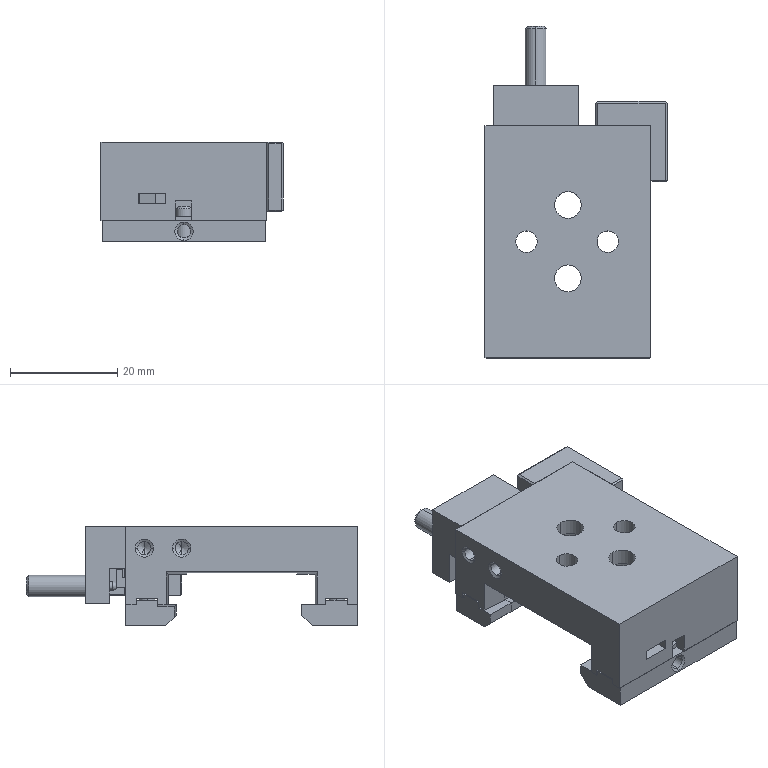Part | NX | 9 solids | 291 faces | box 34 x 62.005 x 18.65 mm | volume 17401 mm3 | plane 137 | cylinder 95 | cone 58 | sphere 1 | commonest cylinder face diameters 2.5 x47 3.3 x10 3 x8 3.2 x6 4 x6 3.5 x4